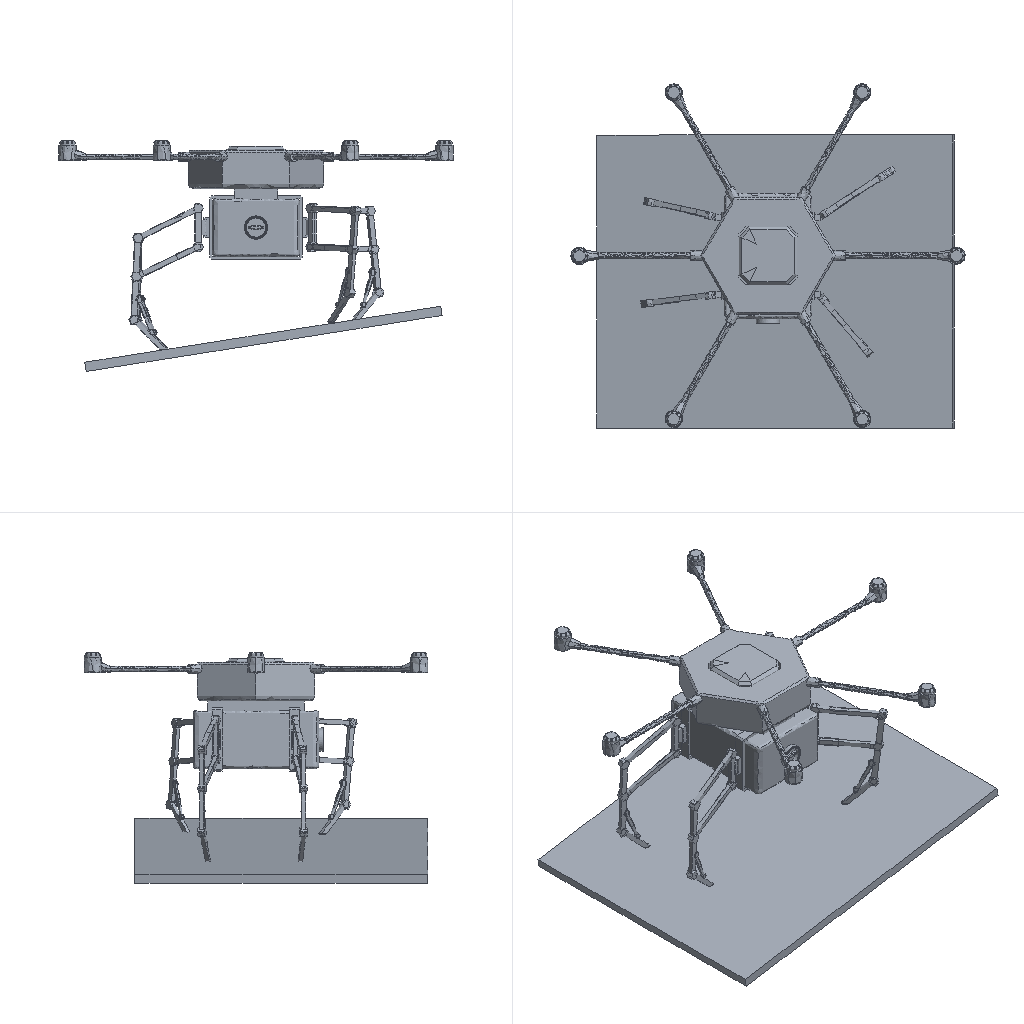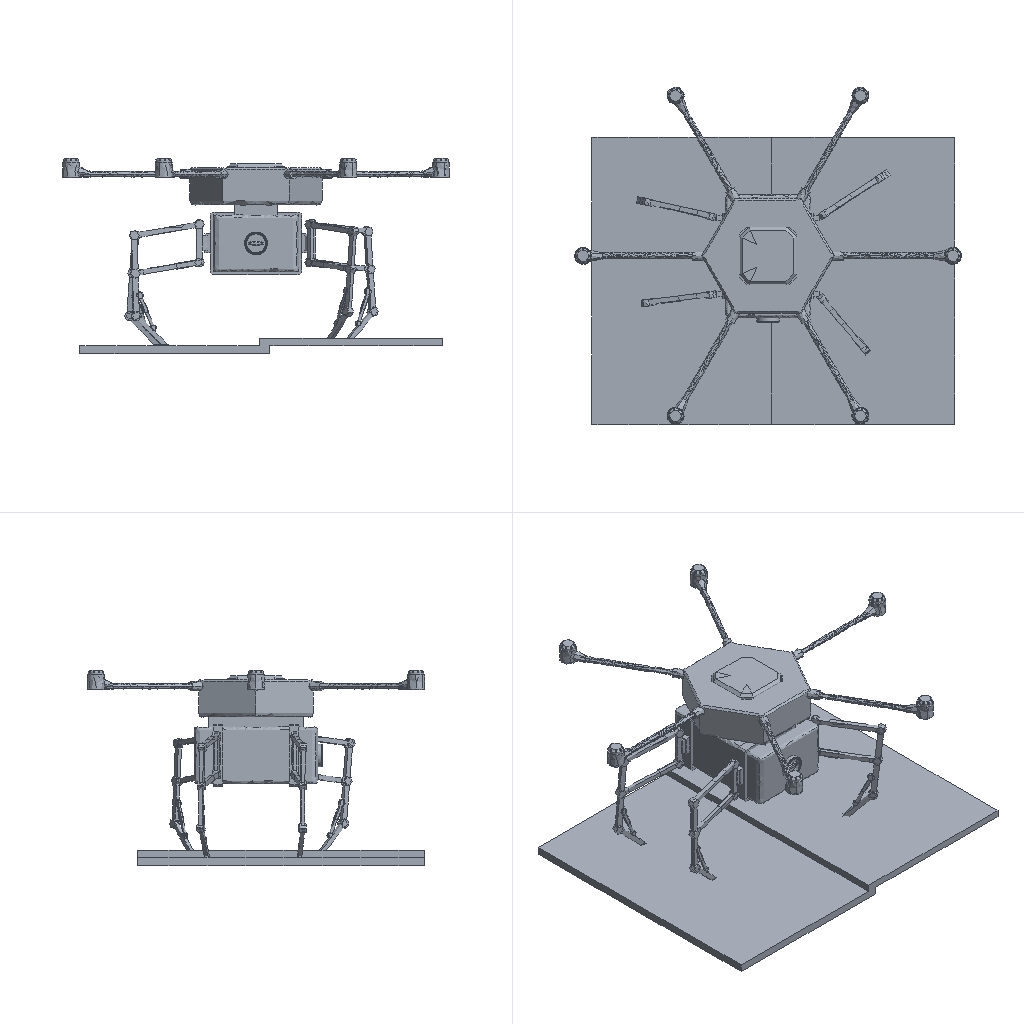Simulation study | ansys workbench
Set-up summary, first 174 of 337 lines:
category,name,step,type,value,unit,region
solver,ansys_workbench
units,mm-N-s-tonne (MPa),,stated,"/units,MPA"
analysis,deck-1/LS1,,static
load_step,deck-1/LS1,deck-1/LS1,static,nsubst=1; time=1
analysis,deck-2/LS1,,static
load_step,deck-2/LS1,deck-2/LS1,static,nsubst=1; time=1
analysis,deck-3/LS1,,static
load_step,deck-3/LS1,deck-3/LS1,static,nsubst=1; time=1
analysis,deck-4/LS1,,transient
load_step,deck-4/LS1,deck-4/LS1,transient,time=1
mesh,deck-1.dat,,nodes,101966
mesh,deck-1.dat,,elements,68262
element_type,SOLID187,,,55120,,deck-1.dat
element_type,TARGE170,,,6347,,deck-1.dat
element_type,CONTA174,,,6347,,deck-1.dat
element_type,SOLID186,,,224,,deck-1.dat
element_type,SURF154,,,224,,deck-1.dat
mesh,deck-2.dat,,nodes,102364
mesh,deck-2.dat,,elements,68991
element_type,SOLID187,,,55341,,deck-2.dat
element_type,TARGE170,,,6353,,deck-2.dat
element_type,CONTA174,,,6353,,deck-2.dat
element_type,SURF154,,,710,,deck-2.dat
element_type,SOLID186,,,234,,deck-2.dat
mesh,deck-3.dat,,nodes,102293
mesh,deck-3.dat,,elements,69065
element_type,SOLID187,,,55351,,deck-3.dat
element_type,TARGE170,,,6424,,deck-3.dat
element_type,CONTA174,,,6424,,deck-3.dat
element_type,SURF154,,,642,,deck-3.dat
element_type,SOLID186,,,224,,deck-3.dat
mesh,deck-4.dat,,nodes,102293
mesh,deck-4.dat,,elements,69065
element_type,SOLID187,,,55351,,deck-4.dat
element_type,TARGE170,,,6424,,deck-4.dat
element_type,CONTA174,,,6424,,deck-4.dat
element_type,SURF154,,,642,,deck-4.dat
element_type,SOLID186,,,224,,deck-4.dat
material,Structural Steel,,E,200000,tonne s^-2 mm^-1
material,Structural Steel,,nu,0.3
material,Structural Steel,,density,7.85e-09,tonne mm^-3
material,Structural Steel,,conductivity,60.5,tonne mm s^-3 C^-1
material,Structural Steel,,specific_heat,4.34e+08,mm^2 s^-2 C^-1
material,Structural Steel,,cte,1.2e-05,C^-1
material,Structural Steel,,permeability,10000
material,Structural Steel,,resistivity,0.00017,ohm mm
material,Structural Steel,,E,200000,tonne s^-2 mm^-1
material,Structural Steel,,nu,0.3
material,Structural Steel,,density,7.85e-09,tonne mm^-3
material,Structural Steel,,conductivity,60.5,tonne mm s^-3 C^-1
material,Structural Steel,,specific_heat,4.34e+08,mm^2 s^-2 C^-1
material,Structural Steel,,cte,1.2e-05,C^-1
material,Structural Steel,,permeability,10000
material,Structural Steel,,resistivity,0.00017,ohm mm
material,Structural Steel,,E,200000,tonne s^-2 mm^-1
material,Structural Steel,,nu,0.3
material,Structural Steel,,density,7.85e-09,tonne mm^-3
material,Structural Steel,,conductivity,60.5,tonne mm s^-3 C^-1
material,Structural Steel,,specific_heat,4.34e+08,mm^2 s^-2 C^-1
material,Structural Steel,,cte,1.2e-05,C^-1
material,Structural Steel,,permeability,10000
material,Structural Steel,,resistivity,0.00017,ohm mm
load,Define Force Using Surface Effect Elements,deck-1/LS1,surface-effect pres face 2,-8.3944e-09,,SURF154 #182
load,Define Force Using Surface Effect Elements,deck-1/LS1,surface-effect pres face 3,-14.087,,SURF154 #182
load,Define Force Using Surface Effect Elements,deck-2/LS1,surface-effect pres face 3,-23.308,,SURF154 #182
load,Define Force Using Surface Effect Elements,deck-3/LS1,surface-effect pres face 3,-2.328,,SURF154 #190
load,Define Force Using Surface Effect Elements,deck-4/LS1,surface-effect pres face 3,-2.328,,SURF154 #190
load,ACEL,deck-4/LS1,gravity (ACEL; gravity acts opposite),"84.28 [dir=(0, 0, 1)]",,all
bc,Fixed Supports,deck-1/model,fixed,[dofs=ALL],,_FIXEDSU
bc,Fixed Supports,deck-2/model,fixed,[dofs=ALL],,_FIXEDSU
bc,Fixed Supports,deck-3/model,fixed,[dofs=ALL],,_FIXEDSU
bc,Fixed Supports,deck-4/model,fixed,[dofs=ALL],,_FIXEDSU
contact,Contact Region,,bonded (always),element=CONTA174
contact,Contact Region 2,,bonded (always),element=CONTA174
contact,Contact Region 3,,bonded (always),element=CONTA174
contact,Contact Region 8,,bonded (always),element=CONTA174
contact,Contact Region 9,,bonded (always),element=CONTA174
contact,Contact Region 10,,bonded (always),element=CONTA174
contact,Contact Region 15,,bonded (always),element=CONTA174
contact,Contact Region 16,,bonded (always),element=CONTA174
contact,Contact Region 17,,bonded (always),element=CONTA174
contact,Contact Region 22,,bonded (always),element=CONTA174
contact,Contact Region 23,,bonded (always),element=CONTA174
contact,Contact Region 24,,bonded (always),element=CONTA174
contact,Contact Region 29,,bonded (always),element=CONTA174
contact,Contact Region 30,,bonded (always),element=CONTA174
contact,Contact Region 31,,bonded (always),element=CONTA174
contact,Contact Region 36,,bonded (always),element=CONTA174
contact,Contact Region 37,,bonded (always),element=CONTA174
contact,Contact Region 38,,bonded (always),element=CONTA174
contact,Contact Region 43,,bonded (always),element=CONTA174
contact,Contact Region 44,,bonded (always),element=CONTA174
contact,Contact Region 45,,bonded (always),element=CONTA174
contact,Contact Region 46,,bonded (always),element=CONTA174
contact,Contact Region 47,,bonded (always),element=CONTA174
contact,Contact Region 48,,bonded (always),element=CONTA174
contact,Contact Region 49,,bonded (always),element=CONTA174
contact,Contact Region 50,,bonded (always),element=CONTA174
contact,Contact Region 51,,bonded (always),element=CONTA174
contact,Contact Region 52,,bonded (always),element=CONTA174
contact,Contact Region 53,,bonded (always),element=CONTA174
contact,Contact Region 54,,bonded (always),element=CONTA174
contact,Contact Region 55,,bonded (always),element=CONTA174
contact,Contact Region 56,,bonded (always),element=CONTA174
contact,Contact Region 57,,bonded (always),element=CONTA174
contact,Contact Region 58,,bonded (always),element=CONTA174
contact,Contact Region 59,,bonded (always),element=CONTA174
contact,Contact Region 60,,bonded (always),element=CONTA174
contact,Contact Region 61,,bonded (always),element=CONTA174
contact,Contact Region 62,,bonded (always),element=CONTA174
contact,Contact Region 63,,bonded (always),element=CONTA174
contact,Contact Region 64,,bonded (always),element=CONTA174
contact,Contact Region 65,,bonded (always),element=CONTA174
contact,Contact Region 66,,bonded (always),element=CONTA174
contact,Contact Region 67,,bonded (always),element=CONTA174
contact,Contact Region 68,,bonded (always),element=CONTA174
contact,Contact Region 69,,bonded (always),element=CONTA174
contact,Contact Region 70,,bonded (always),element=CONTA174
contact,Contact Region 71,,bonded (always),element=CONTA174
contact,Contact Region 72,,bonded (always),element=CONTA174
contact,Contact Region 73,,bonded (always),element=CONTA174
contact,Contact Region 74,,bonded (always),element=CONTA174
contact,Contact Region 75,,bonded (always),element=CONTA174
contact,Contact Region 76,,bonded (always),element=CONTA174
contact,Contact Region 77,,bonded (always),element=CONTA174
contact,Contact Region 78,,bonded (always),element=CONTA174
contact,Contact Region 79,,bonded (always),element=CONTA174
contact,Contact Region 80,,bonded (always),element=CONTA174
contact,Contact Region 81,,bonded (always),element=CONTA174
contact,Contact Region 82,,bonded (always),element=CONTA174
contact,Contact Region 83,,bonded (always),element=CONTA174
contact,Contact Region 84,,bonded (always),element=CONTA174
contact,Contact Region 85,,bonded (always),element=CONTA174
contact,Contact Region 86,,bonded (always),element=CONTA174
contact,Contact Region 87,,bonded (always),element=CONTA174
contact,Contact Region,,bonded (always),element=CONTA174
contact,Contact Region 2,,bonded (always),element=CONTA174
contact,Contact Region 3,,bonded (always),element=CONTA174
contact,Contact Region 8,,bonded (always),element=CONTA174
contact,Contact Region 9,,bonded (always),element=CONTA174
contact,Contact Region 10,,bonded (always),element=CONTA174
contact,Contact Region 15,,bonded (always),element=CONTA174
contact,Contact Region 16,,bonded (always),element=CONTA174
contact,Contact Region 17,,bonded (always),element=CONTA174
contact,Contact Region 22,,bonded (always),element=CONTA174
contact,Contact Region 23,,bonded (always),element=CONTA174
contact,Contact Region 24,,bonded (always),element=CONTA174
contact,Contact Region 29,,bonded (always),element=CONTA174
contact,Contact Region 30,,bonded (always),element=CONTA174
contact,Contact Region 31,,bonded (always),element=CONTA174
contact,Contact Region 36,,bonded (always),element=CONTA174
contact,Contact Region 37,,bonded (always),element=CONTA174
contact,Contact Region 38,,bonded (always),element=CONTA174
contact,Contact Region 43,,bonded (always),element=CONTA174
contact,Contact Region 44,,bonded (always),element=CONTA174
contact,Contact Region 45,,bonded (always),element=CONTA174
contact,Contact Region 46,,bonded (always),element=CONTA174
contact,Contact Region 47,,bonded (always),element=CONTA174
contact,Contact Region 48,,bonded (always),element=CONTA174
contact,Contact Region 49,,bonded (always),element=CONTA174
contact,Contact Region 50,,bonded (always),element=CONTA174
contact,Contact Region 51,,bonded (always),element=CONTA174
contact,Contact Region 52,,bonded (always),element=CONTA174
contact,Contact Region 53,,bonded (always),element=CONTA174
contact,Contact Region 54,,bonded (always),element=CONTA174
contact,Contact Region 55,,bonded (always),element=CONTA174
contact,Contact Region 56,,bonded (always),element=CONTA174
contact,Contact Region 57,,bonded (always),element=CONTA174
contact,Contact Region 58,,bonded (always),element=CONTA174
contact,Contact Region 59,,bonded (always),element=CONTA174
contact,Contact Region 60,,bonded (always),element=CONTA174
contact,Contact Region 61,,bonded (always),element=CONTA174
contact,Contact Region 62,,bonded (always),element=CONTA174
Results summary:
result,analyses[0].index,,,1
result,analyses[0].system,,,SYS
result,analyses[0].deck,,,deck-1.dat
result,analyses[0].solve_status,,,completed
result,analyses[0].analysis_type,,,static
result,analyses[0].physics,,,mechanical
result,analyses[0].unit_system,,,"NMM: mm, ton, N, s, mV, mA, degC"
result,analyses[0].n_sets,,,1
result,analyses[0].load_steps[0].set,set=1,,1
result,analyses[0].load_steps[0].time_or_freq,set=1,,1
result,analyses[0].load_steps[0].max_displacement_magnitude,set=1,,0.03028
result,analyses[0].load_steps[0].max_von_mises_nodal,set=1,,73.515
result,analyses[0].load_steps[0].reaction_force_sum_xyz[1],set=1,,-0.06083
result,analyses[0].load_steps[0].reaction_force_sum_xyz[2],set=1,,-0.04394
result,analyses[0].load_steps[0].reaction_force_sum_xyz[3],set=1,,5e+06
result,analyses[1].index,,,2
result,analyses[1].system,,,SYS-1
result,analyses[1].deck,,,deck-2.dat
result,analyses[1].solve_status,,,completed
result,analyses[1].analysis_type,,,static
result,analyses[1].physics,,,mechanical
result,analyses[1].unit_system,,,"NMM: mm, ton, N, s, mV, mA, degC"
result,analyses[1].n_sets,,,1
result,analyses[1].load_steps[0].set,set=1,,1
result,analyses[1].load_steps[0].time_or_freq,set=1,,1
result,analyses[1].load_steps[0].max_displacement_magnitude,set=1,,0.0501
result,analyses[1].load_steps[0].max_von_mises_nodal,set=1,,180.977
result,analyses[1].load_steps[0].reaction_force_sum_xyz[1],set=1,,-0.02836
result,analyses[1].load_steps[0].reaction_force_sum_xyz[2],set=1,,-0.01772
result,analyses[1].load_steps[0].reaction_force_sum_xyz[3],set=1,,5e+07
result,analyses[2].index,,,3
result,analyses[2].system,,,SYS-2
result,analyses[2].deck,,,deck-3.dat
result,analyses[2].solve_status,,,completed
result,analyses[2].analysis_type,,,static
result,analyses[2].physics,,,mechanical
result,analyses[2].unit_system,,,"NMM: mm, ton, N, s, mV, mA, degC"
result,analyses[2].n_sets,,,1
result,analyses[2].load_steps[0].set,set=1,,1
result,analyses[2].load_steps[0].time_or_freq,set=1,,1
result,analyses[2].load_steps[0].max_displacement_magnitude,set=1,,0.004044
result,analyses[2].load_steps[0].max_von_mises_nodal,set=1,,18.183
result,analyses[2].load_steps[0].reaction_force_sum_xyz[1],set=1,,-0.01043
result,analyses[2].load_steps[0].reaction_force_sum_xyz[2],set=1,,-0.001494
result,analyses[2].load_steps[0].reaction_force_sum_xyz[3],set=1,,5e+06
result,analyses[3].index,,,4
result,analyses[3].system,,,SYS-3
result,analyses[3].deck,,,deck-4.dat
result,analyses[3].solve_status,,,completed
result,analyses[3].analysis_type,,,static
result,analyses[3].physics,,,mechanical
result,analyses[3].unit_system,,,"NMM: mm, ton, N, s, mV, mA, degC"
result,analyses[3].n_sets,,,1
result,analyses[3].load_steps[0].set,set=1,,1
result,analyses[3].load_steps[0].time_or_freq,set=1,,1
result,analyses[3].load_steps[0].max_displacement_magnitude,set=1,,0.004602
result,analyses[3].load_steps[0].max_von_mises_nodal,set=1,,22.16
result,analyses[3].load_steps[0].reaction_force_sum_xyz[1],set=1,,-0.0005344
result,analyses[3].load_steps[0].reaction_force_sum_xyz[2],set=1,,3.36593e-05
result,analyses[3].load_steps[0].reaction_force_sum_xyz[3],set=1,,4.99814e+06